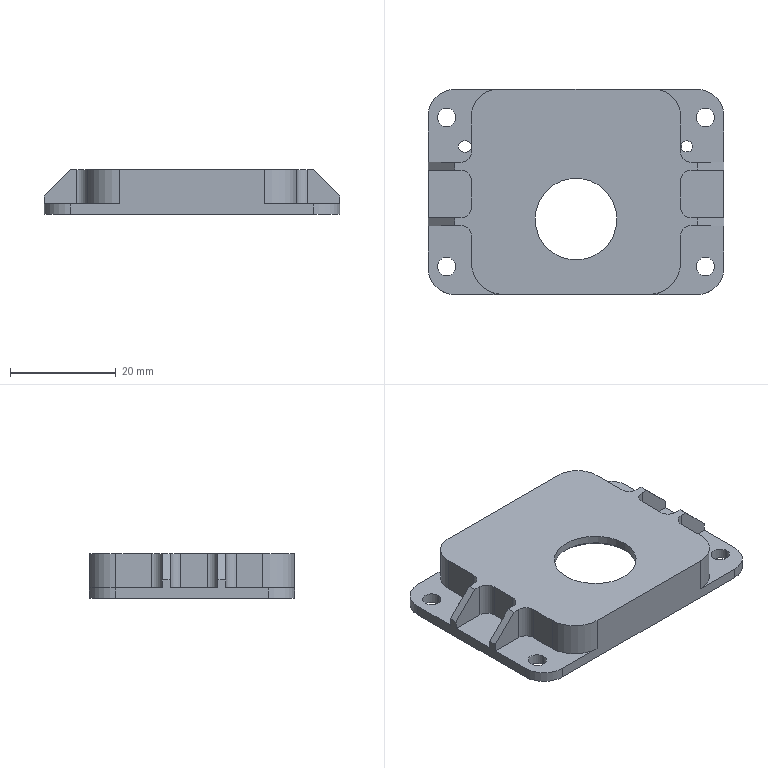NC program | NX | posted with a generic post | part box 56 x 38.85 x 8.5 mm
Lines 1051 to 2659 of 4316:
(CAVITY_MILL_COPY , TOOL : D4)
N2082 T11 M6
N2084 G54
N2086 G17 G0 G90 X-22.6 Y-12.105 S9500 M3
N2088 G43 Z30. H11
N2090 Z0.618
N2092 G94 G1 Z-0.382 F1000.
N2094 X-22.3 Y-11.932
N2096 G3 X-21.8 Y-11.066 R1.
N2098 G1 Y-8.375 F1400.
N2100 X-23.382
N2102 G2 X-24.06 Y-8.257 R2.
N2104 G3 X-25.044 Y-8.434 R1.
N2106 G1 X-25.164 Y-8.535
N2108 Z0.618
N2110 G0 Z30.
N2112 X-22.6 Y-12.201
N2114 Z0.235
N2116 G1 Z-0.765 F1000.
N2118 X-22.3 Y-12.028
N2120 G3 X-21.8 Y-11.162 R1.
N2122 G1 Y-8.375 F1400.
N2124 X-23.765
N2126 G2 X-24.289 Y-8.301 R2.016
N2128 G3 X-25.257 Y-8.551 R1.
N2130 G1 X-25.37 Y-8.662
N2132 Z0.235
N2134 G0 X-22.6 Y-12.258 Z-0.147
N2136 G1 Z-1.147 F1000.
N2138 X-22.3 Y-12.084
N2140 G3 X-21.8 Y-11.218 R1.
N2142 G1 Y-8.375 F1400.
N2144 X-24.147
N2146 G2 X-24.473 Y-8.346 R2.015
N2148 G3 X-25.411 Y-8.693 R1.
N2150 G1 X-25.512 Y-8.814
N2152 Z-0.147
N2154 G0 X-22.6 Y-12.301 Z-0.529
N2156 G1 Z-1.529 F1000.
N2158 X-22.3 Y-12.127
N2160 G3 X-21.8 Y-11.261 R1.
N2162 G1 Y-8.375 F1400.
N2164 X-24.529
N2166 X-24.647 Y-8.372
N2168 G3 X-25.541 Y-8.82 R1.
N2170 G1 X-25.627 Y-8.951
N2172 Z-0.529
N2174 G0 X-22.6 Y-12.311 Z-0.912
N2176 G1 Z-1.912 F1000.
N2178 X-22.3 Y-12.138
N2180 G3 X-21.8 Y-11.272 R1.
N2182 G1 Y-8.375 F1400.
N2184 X-24.697
N2186 G3 X-25.563 Y-8.875 R1.
N2188 G1 X-25.675 Y-9.069
N2190 Z-0.912
N2192 G0 X-22.6 Y-12.311 Z-1.294
N2194 G1 Z-2.294 F1000.
N2196 X-22.3 Y-12.138
N2198 G3 X-21.8 Y-11.272 R1.
N2200 G1 Y-8.375 F1400.
N2202 X-24.697
N2204 G3 X-25.563 Y-8.875 R1.
N2206 G1 X-25.716 Y-9.141
N2208 Z-1.294
N2210 G0 X-22.6 Y-12.311 Z-1.676
N2212 G1 Z-2.676 F1000.
N2214 X-22.3 Y-12.138
N2216 G3 X-21.8 Y-11.272 R1.
N2218 G1 Y-8.375 F1400.
N2220 X-24.697
N2222 G3 X-25.563 Y-8.875 R1.
N2224 G1 X-25.736 Y-9.174
N2226 Z-1.676
N2228 G0 X-22.6 Y-12.311 Z-2.059
N2230 G1 Z-3.059 F1000.
N2232 X-22.3 Y-12.138
N2234 G3 X-21.8 Y-11.272 R1.
N2236 G1 Y-8.375 F1400.
N2238 X-24.697
N2240 G3 X-25.563 Y-8.875 R1.
N2242 G1 X-25.736 Y-9.175
N2244 Z-2.059
N2246 G0 X-22.6 Y-12.311 Z-2.441
N2248 G1 Z-3.441 F1000.
N2250 X-22.3 Y-12.138
N2252 G3 X-21.8 Y-11.272 R1.
N2254 G1 Y-8.375 F1400.
N2256 X-24.697
N2258 G3 X-25.563 Y-8.875 R1.
N2260 G1 X-25.736 Y-9.175
N2262 Z-2.441
N2264 G0 X-22.6 Y-12.311 Z-2.824
N2266 G1 Z-3.824 F1000.
N2268 X-22.3 Y-12.138
N2270 G3 X-21.8 Y-11.272 R1.
N2272 G1 Y-8.375 F1400.
N2274 X-24.697
N2276 G3 X-25.563 Y-8.875 R1.
N2278 G1 X-25.736 Y-9.175
N2280 Z-2.824
N2282 G0 X-22.6 Y-12.311 Z-3.206
N2284 G1 Z-4.206 F1000.
N2286 X-22.3 Y-12.138
N2288 G3 X-21.8 Y-11.272 R1.
N2290 G1 Y-8.375 F1400.
N2292 X-24.697
N2294 G3 X-25.563 Y-8.875 R1.
N2296 G1 X-25.736 Y-9.175
N2298 Z-3.206
N2300 G0 X-22.6 Y-12.311 Z-3.588
N2302 G1 Z-4.588 F1000.
N2304 X-22.3 Y-12.138
N2306 G3 X-21.8 Y-11.272 R1.
N2308 G1 Y-8.375 F1400.
N2310 X-24.697
N2312 G3 X-25.563 Y-8.875 R1.
N2314 G1 X-25.736 Y-9.175
N2316 Z-3.588
N2318 G0 X-22.6 Y-12.311 Z-3.971
N2320 G1 Z-4.971 F1000.
N2322 X-22.3 Y-12.138
N2324 G3 X-21.8 Y-11.272 R1.
N2326 G1 Y-8.375 F1400.
N2328 X-24.697
N2330 G3 X-25.563 Y-8.875 R1.
N2332 G1 X-25.736 Y-9.175
N2334 Z-3.971
N2336 G0 X-22.6 Y-12.311 Z-4.353
N2338 G1 Z-5.353 F1000.
N2340 X-22.3 Y-12.138
N2342 G3 X-21.8 Y-11.272 R1.
N2344 G1 Y-8.375 F1400.
N2346 X-24.697
N2348 G3 X-25.563 Y-8.875 R1.
N2350 G1 X-25.736 Y-9.175
N2352 Z-4.353
N2354 G0 X-22.6 Y-12.311 Z-4.735
N2356 G1 Z-5.735 F1000.
N2358 X-22.3 Y-12.138
N2360 G3 X-21.8 Y-11.272 R1.
N2362 G1 Y-8.375 F1400.
N2364 X-24.697
N2366 G3 X-25.563 Y-8.875 R1.
N2368 G1 X-25.736 Y-9.175
N2370 Z-4.735
N2372 G0 X-22.6 Y-12.311 Z-5.118
N2374 G1 Z-6.118 F1000.
N2376 X-22.3 Y-12.138
N2378 G3 X-21.8 Y-11.272 R1.
N2380 G1 Y-8.375 F1400.
N2382 X-24.697
N2384 G3 X-25.563 Y-8.875 R1.
N2386 G1 X-25.736 Y-9.175
N2388 Z-5.118
N2390 G0 X-22.6 Y-12.311 Z-5.5
N2392 G1 Z-6.5 F1000.
N2394 X-22.3 Y-12.138
N2396 G3 X-21.8 Y-11.272 R1.
N2398 G1 Y-8.375 F1400.
N2400 X-24.697
N2402 G3 X-25.563 Y-8.875 R1.
N2404 G1 X-25.736 Y-9.175
N2406 Z-5.5
N2408 G0 Z30.
N2410 X-25.495 Y-3.037
N2412 Z0.618
N2414 G1 Z-0.382 F1000.
N2416 X-25.36 Y-3.118
N2418 G3 X-24.36 Y-3.13 R1.
N2420 G2 X-23.382 Y-2.875 R2. F1400.
N2422 G1 X-21.8
N2424 Y2.125
N2426 X-23.382
N2428 G2 X-24.361 Y2.381 R2.
N2430 G3 X-25.361 Y2.369 R1.
N2432 G1 X-25.496 Y2.289
N2434 Z0.618
N2436 G0 Z30.
N2438 X-25.877 Y-3.037
N2440 Z0.235
N2442 G1 Z-0.765 F1000.
N2444 X-25.742 Y-3.118
N2446 G3 X-24.742 Y-3.13 R1.
N2448 G2 X-23.765 Y-2.875 R2. F1400.
N2450 G1 X-21.8
N2452 Y2.125
N2454 X-23.765
N2456 G2 X-24.744 Y2.381 R2.
N2458 G3 X-25.744 Y2.369 R1.
N2460 G1 X-25.878 Y2.289
N2462 Z0.235
N2464 G0 X-25.545 Y1.215 Z-0.147
N2466 G1 Z-1.147 F1000.
N2468 X-24.284 Y0.498
N2470 G2 X-23.779 Y-0.365 R1.
N2472 X-24.94 Y-2.525 R2.56 F1400.
N2474 G3 X-25.129 Y-3.133 R0.5
N2476 G2 X-24.147 Y-2.875 R2.
N2478 G1 X-21.8
N2480 Y2.125
N2482 X-24.147
N2484 G2 X-25.159 Y2.4 R2.
N2486 G3 X-24.967 Y1.781 R0.5
N2488 G2 X-23.779 Y-0.365 R2.56
N2490 X-24.273 Y-1.234 R1.
N2492 G1 X-25.524 Y-1.967
N2494 Z-0.147
N2496 G0 X-25.927 Y1.215 Z-0.529
N2498 G1 Z-1.529 F1000.
N2500 X-24.666 Y0.496
N2502 G2 X-24.161 Y-0.367 R1.
N2504 X-25.322 Y-2.525 R2.56 F1400.
N2506 G3 X-25.512 Y-3.133 R0.5
N2508 G2 X-24.529 Y-2.875 R2.
N2510 G1 X-21.8
N2512 Y2.125
N2514 X-24.529
N2516 G2 X-25.541 Y2.4 R2.
N2518 G3 X-25.35 Y1.781 R0.5
N2520 G2 X-24.161 Y-0.367 R2.56
N2522 X-24.656 Y-1.236 R1.
N2524 G1 X-25.906 Y-1.967
N2526 Z-0.529
N2528 G0 X-26.31 Y1.216 Z-0.912
N2530 G1 Z-1.912 F1000.
N2532 X-25.048 Y0.495
N2534 G2 X-24.544 Y-0.369 R1.
N2536 X-25.705 Y-2.525 R2.56 F1400.
N2538 G3 X-25.894 Y-3.133 R0.5
N2540 G2 X-24.912 Y-2.875 R2.
N2542 G1 X-21.8
N2544 Y2.125
N2546 X-24.912
N2548 G2 X-25.924 Y2.4 R2.
N2550 G3 X-25.732 Y1.781 R0.5
N2552 G2 X-24.544 Y-0.369 R2.56
N2554 X-25.039 Y-1.237 R1.
N2556 G1 X-26.289 Y-1.966
N2558 Z-0.912
N2560 G0 X-26.693 Y1.216 Z-1.294
N2562 G1 Z-2.294 F1000.
N2564 X-25.43 Y0.494
N2566 G2 X-24.926 Y-0.37 R1.
N2568 X-26.087 Y-2.525 R2.56 F1400.
N2570 G3 X-26.276 Y-3.133 R0.5
N2572 G2 X-25.294 Y-2.875 R2.
N2574 G1 X-21.8
N2576 Y2.125
N2578 X-25.294
N2580 G2 X-26.306 Y2.4 R2.
N2582 G3 X-26.114 Y1.781 R0.5
N2584 G2 X-24.926 Y-0.37 R2.56
N2586 X-25.422 Y-1.238 R1.
N2588 G1 X-26.671 Y-1.966
N2590 Z-1.294
N2592 G0 X-27.075 Y1.216 Z-1.676
N2594 G1 Z-2.676 F1000.
N2596 X-25.811 Y0.493
N2598 G2 X-25.308 Y-0.372 R1.
N2600 X-26.469 Y-2.525 R2.56 F1400.
N2602 G3 X-26.659 Y-3.133 R0.5
N2604 G2 X-25.676 Y-2.875 R2.
N2606 G1 X-21.8
N2608 Y2.125
N2610 X-25.676
N2612 G2 X-26.688 Y2.4 R2.
N2614 G3 X-26.497 Y1.781 R0.5
N2616 G2 X-25.308 Y-0.372 R2.56
N2618 X-25.805 Y-1.239 R1.
N2620 G1 X-27.053 Y-1.966
N2622 Z-1.676
N2624 G0 X-27.448 Y-1.973 Z-2.059
N2626 G1 Z-3.059 F1000.
N2628 X-26.188 Y-1.24
N2630 G3 X-25.691 Y-0.373 R1.
N2632 G1 X-23.891 Y-0.367
N2634 G2 X-23.946 Y-1.075 R4.36 F1400.
N2636 G1 X-23.6
N2638 Y0.325
N2640 X-23.948
N2642 G2 X-23.891 Y-0.367 R4.36
N2644 G1 X-25.691 Y-0.373
N2646 G2 X-26.866 Y-2.534 R2.56
N2648 G3 X-27.055 Y-3.151 R0.5
N2650 G2 X-26.007 Y-2.875 R2.026
N2652 G1 X-21.8
N2654 Y2.125
N2656 X-26.029
N2658 G2 X-27.08 Y2.412 R2.015
N2660 G3 X-26.888 Y1.786 R0.5
N2662 G2 X-25.691 Y-0.373 R2.56
N2664 X-26.188 Y-1.24 R1.
N2666 G1 X-27.448 Y-1.973
N2668 Z-2.059
N2670 G0 X-27.817 Y-1.965 Z-2.441
N2672 G1 Z-3.441 F1000.
N2674 X-26.572 Y-1.244
N2676 G3 X-26.073 Y-0.377 R1.
N2678 G1 X-24.273 Y-0.375
N2680 G2 X-24.329 Y-1.075 R4.36 F1400.
N2682 G1 X-23.6
N2684 Y0.325
N2686 X-24.331
N2688 G2 X-24.273 Y-0.375 R4.36
N2690 G1 X-26.073 Y-0.377
N2692 G2 X-27.234 Y-2.525 R2.56
N2694 G3 X-27.424 Y-3.133 R0.5
N2696 G2 X-26.441 Y-2.875 R2.
N2698 G1 X-21.8
N2700 Y2.125
N2702 X-26.441
N2704 G2 X-27.453 Y2.4 R2.
N2706 G3 X-27.261 Y1.781 R0.5
N2708 G2 X-26.073 Y-0.377 R2.56
N2710 X-26.572 Y-1.244 R1.
N2712 G1 X-27.817 Y-1.965
N2714 Z-2.441
N2716 G0 X-28.199 Z-2.824
N2718 G1 Z-3.824 F1000.
N2720 X-26.954 Y-1.244
N2722 G3 X-26.455 Y-0.377 R1.
N2724 G1 X-24.655 Y-0.375
N2726 G2 X-24.711 Y-1.075 R4.36 F1400.
N2728 G1 X-23.6
N2730 Y0.325
N2732 X-24.713
N2734 G2 X-24.655 Y-0.375 R4.36
N2736 G1 X-26.455 Y-0.377
N2738 G2 X-27.616 Y-2.525 R2.56
N2740 G3 X-27.806 Y-3.133 R0.5
N2742 G2 X-26.824 Y-2.875 R2.
N2744 G1 X-21.8
N2746 Y2.125
N2748 X-26.824
N2750 G2 X-27.835 Y2.4 R2.
N2752 G3 X-27.644 Y1.781 R0.5
N2754 G2 X-26.455 Y-0.377 R2.56
N2756 X-26.954 Y-1.244 R1.
N2758 G1 X-28.199 Y-1.965
N2760 Z-2.824
N2762 G0 X-28.581 Z-3.206
N2764 G1 Z-4.206 F1000.
N2766 X-27.337 Y-1.245
N2768 G3 X-26.838 Y-0.378 R1.
N2770 G1 X-24.438 Y-0.375
N2772 X-24.439 Y-0.475 F1400.
N2774 X-24.2
N2776 Y-0.275
N2778 X-24.439
N2780 X-24.438 Y-0.375
N2782 X-26.838 Y-0.378
N2784 Y-0.43
N2786 G2 X-27.999 Y-2.525 R2.56
N2788 G3 X-28.188 Y-3.133 R0.5
N2790 G2 X-27.206 Y-2.875 R2.
N2792 G1 X-21.8
N2794 Y2.125
N2796 X-27.206
N2798 G2 X-28.218 Y2.4 R2.
N2800 G3 X-28.026 Y1.781 R0.5
N2802 G2 X-26.838 Y-0.378 R2.56
N2804 X-27.337 Y-1.245 R1.
N2806 G1 X-28.581 Y-1.965
N2808 Z-3.206
N2810 G0 X-28.964 Z-3.588
N2812 G1 Z-4.588 F1000.
N2814 X-27.719 Y-1.245
N2816 G3 X-27.22 Y-0.378 R1.
N2818 G1 X-24.82 Y-0.375
N2820 X-24.821 Y-0.475 F1400.
N2822 X-24.2
N2824 Y-0.275
N2826 X-24.821
N2828 X-24.82 Y-0.375
N2830 X-27.22 Y-0.378
N2832 Y-0.43
N2834 G2 X-28.381 Y-2.525 R2.56
N2836 G3 X-28.571 Y-3.133 R0.5
N2838 G2 X-27.588 Y-2.875 R2.
N2840 G1 X-21.8
N2842 Y2.125
N2844 X-27.588
N2846 G2 X-28.6 Y2.4 R2.
N2848 G3 X-28.409 Y1.781 R0.5
N2850 G2 X-27.22 Y-0.378 R2.56
N2852 X-27.719 Y-1.245 R1.
N2854 G1 X-28.964 Y-1.965
N2856 Z-3.588
N2858 G0 X-29.347 Y-1.966 Z-3.971
N2860 G1 Z-4.971 F1000.
N2862 X-28.103 Y-1.245
N2864 G3 X-27.604 Y-0.378 R1.
N2866 G1 X-25.204 Y-0.375
N2868 X-25.205 Y-0.475 F1400.
N2870 X-24.2
N2872 Y-0.275
N2874 X-25.206
N2876 X-25.204 Y-0.375
N2878 X-27.604 Y-0.378
N2880 X-27.605 Y-0.43
N2882 G2 X-28.764 Y-2.525 R2.56
N2884 G3 X-28.954 Y-3.133 R0.5
N2886 G2 X-27.971 Y-2.875 R2.
N2888 G1 X-21.8
N2890 Y2.125
N2892 X-27.971
N2894 G2 X-28.958 Y2.386 R2.
N2896 G3 X-28.772 Y1.778 R0.5
N2898 G2 X-28.136 Y1.18 R2.56
N2900 X-27.604 Y-0.378 R2.56
N2902 X-28.103 Y-1.245 R1.
N2904 G1 X-29.347 Y-1.966
N2906 Z-3.971
N2908 G0 X-29.384 Y-1.969 Z-4.353
N2910 G1 Z-5.353 F1000.
N2912 X-28.143 Y-1.248
N2914 G3 X-27.645 Y-0.381 R1.
N2916 G1 X-25.245 Y-0.375
N2918 X-25.246 Y-0.475 F1400.
N2920 X-24.2
N2922 Y-0.275
N2924 X-25.247
N2926 X-25.245 Y-0.375
N2928 X-27.645 Y-0.381
N2930 X-27.646 Y-0.433
N2932 G2 X-28.8 Y-2.527 R2.56
N2934 G3 X-28.988 Y-3.136 R0.5
N2936 G2 X-28. Y-2.875 R2.
N2938 G1 X-21.8
N2940 Y2.125
N2942 X-28.
N2944 G2 X-29.02 Y2.404 R2.
N2946 G3 X-28.843 Y1.793 R0.5
N2948 G2 X-28.677 Y1.669 R2.56
N2950 G1 X-28.595 Y1.602
N2952 G2 X-27.645 Y-0.381 R2.56
N2954 X-28.143 Y-1.248 R1.
N2956 G1 X-29.384 Y-1.969
N2958 Z-4.353
N2960 G0 Z-4.735
N2962 G1 Z-5.735 F1000.
N2964 X-28.143 Y-1.248
N2966 G3 X-27.645 Y-0.381 R1.
N2968 G1 X-25.245 Y-0.375
N2970 X-25.246 Y-0.475 F1400.
N2972 X-24.2
N2974 Y-0.275
N2976 X-25.247
N2978 X-25.245 Y-0.375
N2980 X-27.645 Y-0.381
N2982 X-27.646 Y-0.433
N2984 G2 X-28.8 Y-2.527 R2.56
N2986 G3 X-28.988 Y-3.136 R0.5
N2988 G2 X-28. Y-2.875 R2.
N2990 G1 X-21.8
N2992 Y2.125
N2994 X-28.
N2996 G2 X-29.02 Y2.404 R2.
N2998 G3 X-28.843 Y1.793 R0.5
N3000 G2 X-28.677 Y1.669 R2.56
N3002 G1 X-28.595 Y1.602
N3004 G2 X-27.645 Y-0.381 R2.56
N3006 X-28.143 Y-1.248 R1.
N3008 G1 X-29.384 Y-1.969
N3010 Z-4.735
N3012 G0 Z-5.118
N3014 G1 Z-6.118 F1000.
N3016 X-28.143 Y-1.248
N3018 G3 X-27.645 Y-0.381 R1.
N3020 G1 X-25.245 Y-0.375
N3022 X-25.246 Y-0.475 F1400.
N3024 X-24.2
N3026 Y-0.275
N3028 X-25.247
N3030 X-25.245 Y-0.375
N3032 X-27.645 Y-0.381
N3034 X-27.646 Y-0.433
N3036 G2 X-28.8 Y-2.527 R2.56
N3038 G3 X-28.988 Y-3.136 R0.5
N3040 G2 X-28. Y-2.875 R2.
N3042 G1 X-21.8
N3044 Y2.125
N3046 X-28.
N3048 G2 X-29.02 Y2.404 R2.
N3050 G3 X-28.843 Y1.793 R0.5
N3052 G2 X-28.677 Y1.669 R2.56
N3054 G1 X-28.595 Y1.602
N3056 G2 X-27.645 Y-0.381 R2.56
N3058 X-28.143 Y-1.248 R1.
N3060 G1 X-29.384 Y-1.969
N3062 Z-5.118
N3064 G0 Z-5.5
N3066 G1 Z-6.5 F1000.
N3068 X-28.143 Y-1.248
N3070 G3 X-27.645 Y-0.381 R1.
N3072 G1 X-25.245 Y-0.375
N3074 X-25.246 Y-0.475 F1400.
N3076 X-24.2
N3078 Y-0.275
N3080 X-25.247
N3082 X-25.245 Y-0.375
N3084 X-27.645 Y-0.381
N3086 X-27.646 Y-0.433
N3088 G2 X-28.8 Y-2.527 R2.56
N3090 G3 X-28.988 Y-3.136 R0.5
N3092 G2 X-28. Y-2.875 R2.
N3094 G1 X-21.8
N3096 Y2.125
N3098 X-28.
N3100 G2 X-29.02 Y2.404 R2.
N3102 G3 X-28.843 Y1.793 R0.5
N3104 G2 X-28.677 Y1.669 R2.56
N3106 G1 X-28.595 Y1.602
N3108 G2 X-27.645 Y-0.381 R2.56
N3110 X-28.143 Y-1.248 R1.
N3112 G1 X-29.384 Y-1.969
N3114 Z-5.5
N3116 G0 Z30.
N3118 X-25.164 Y7.785
N3120 Z0.618
N3122 G1 Z-0.382 F1000.
N3124 X-25.044 Y7.684
N3126 G3 X-24.06 Y7.507 R1.
N3128 G2 X-23.382 Y7.625 R2. F1400.
N3130 G1 X-21.8
N3132 Y10.316
N3134 G3 X-22.3 Y11.182 R1.
N3136 G1 X-22.6 Y11.355
N3138 Z0.618
N3140 G0 Z30.
N3142 X-25.367 Y7.921
N3144 Z0.235
N3146 G1 Z-0.765 F1000.
N3148 X-25.256 Y7.811
N3150 G3 X-24.289 Y7.555 R1.
N3152 G2 X-23.765 Y7.625 R2. F1400.
N3154 G1 X-21.8
N3156 Y10.412
N3158 G3 X-22.3 Y11.278 R1.
N3160 G1 X-22.6 Y11.451
N3162 Z0.235
N3164 G0 X-25.509 Y8.071 Z-0.147
N3166 G1 Z-1.147 F1000.
N3168 X-25.41 Y7.95
N3170 G3 X-24.474 Y7.598 R1.
N3172 G2 X-24.147 Y7.625 R2. F1400.
N3174 G1 X-21.8
N3176 Y10.469
N3178 G3 X-22.3 Y11.335 R1.
N3180 G1 X-22.6 Y11.508
N3182 Z-0.147
N3184 G0 X-25.628 Y8.201 Z-0.529
N3186 G1 Z-1.529 F1000.
N3188 X-25.541 Y8.07
N3190 G3 X-24.647 Y7.622 R1.
N3192 G1 X-24.529 Y7.625 F1400.
N3194 X-21.8
N3196 Y10.512
N3198 G3 X-22.3 Y11.378 R1.
N3200 G1 X-22.6 Y11.551
N3202 Z-0.529
N3204 G0 X-25.675 Y8.319 Z-0.912
N3206 G1 Z-1.912 F1000.
N3208 X-25.563 Y8.125
N3210 G3 X-24.697 Y7.625 R1.
N3212 G1 X-21.8 F1400.
N3214 Y10.522
N3216 G3 X-22.3 Y11.388 R1.
N3218 G1 X-22.6 Y11.561
N3220 Z-0.912
N3222 G0 X-25.718 Y8.393 Z-1.294
N3224 G1 Z-2.294 F1000.
N3226 X-25.563 Y8.125
N3228 G3 X-24.697 Y7.625 R1.
N3230 G1 X-21.8 F1400.
N3232 Y10.522
N3234 G3 X-22.3 Y11.388 R1.
N3236 G1 X-22.6 Y11.561
N3238 Z-1.294
N3240 G0 X-25.736 Y8.424 Z-1.676
N3242 G1 Z-2.676 F1000.
N3244 X-25.563 Y8.125
N3246 G3 X-24.697 Y7.625 R1.
N3248 G1 X-21.8 F1400.
N3250 Y10.522
N3252 G3 X-22.3 Y11.388 R1.
N3254 G1 X-22.6 Y11.561
N3256 Z-1.676
N3258 G0 X-25.736 Y8.425 Z-2.059
N3260 G1 Z-3.059 F1000.
N3262 X-25.563 Y8.125
N3264 G3 X-24.697 Y7.625 R1.
N3266 G1 X-21.8 F1400.
N3268 Y10.522
N3270 G3 X-22.3 Y11.388 R1.
N3272 G1 X-22.6 Y11.561
N3274 Z-2.059
N3276 G0 X-25.736 Y8.425 Z-2.441
N3278 G1 Z-3.441 F1000.
N3280 X-25.563 Y8.125
N3282 G3 X-24.697 Y7.625 R1.
N3284 G1 X-21.8 F1400.
N3286 Y10.522
N3288 G3 X-22.3 Y11.388 R1.
N3290 G1 X-22.6 Y11.561
N3292 Z-2.441
N3294 G0 X-25.736 Y8.425 Z-2.824
N3296 G1 Z-3.824 F1000.
N3298 X-25.563 Y8.125
N3300 G3 X-24.697 Y7.625 R1.
N3302 G1 X-21.8 F1400.
N3304 Y10.522
N3306 G3 X-22.3 Y11.388 R1.
N3308 G1 X-22.6 Y11.561
N3310 Z-2.824
N3312 G0 X-25.736 Y8.425 Z-3.206
N3314 G1 Z-4.206 F1000.
N3316 X-25.563 Y8.125
N3318 G3 X-24.697 Y7.625 R1.
N3320 G1 X-21.8 F1400.
N3322 Y10.522
N3324 G3 X-22.3 Y11.388 R1.
N3326 G1 X-22.6 Y11.561
N3328 Z-3.206
N3330 G0 X-25.736 Y8.425 Z-3.588
N3332 G1 Z-4.588 F1000.
N3334 X-25.563 Y8.125
N3336 G3 X-24.697 Y7.625 R1.
N3338 G1 X-21.8 F1400.
N3340 Y10.522
N3342 G3 X-22.3 Y11.388 R1.
N3344 G1 X-22.6 Y11.561
N3346 Z-3.588
N3348 G0 X-25.736 Y8.425 Z-3.971
N3350 G1 Z-4.971 F1000.
N3352 X-25.563 Y8.125
N3354 G3 X-24.697 Y7.625 R1.
N3356 G1 X-21.8 F1400.
N3358 Y10.522
N3360 G3 X-22.3 Y11.388 R1.
N3362 G1 X-22.6 Y11.561
N3364 Z-3.971
N3366 G0 X-25.736 Y8.425 Z-4.353
N3368 G1 Z-5.353 F1000.
N3370 X-25.563 Y8.125
N3372 G3 X-24.697 Y7.625 R1.
N3374 G1 X-21.8 F1400.
N3376 Y10.522
N3378 G3 X-22.3 Y11.388 R1.
N3380 G1 X-22.6 Y11.561
N3382 Z-4.353
N3384 G0 X-25.736 Y8.425 Z-4.735
N3386 G1 Z-5.735 F1000.
N3388 X-25.563 Y8.125
N3390 G3 X-24.697 Y7.625 R1.
N3392 G1 X-21.8 F1400.
N3394 Y10.522
N3396 G3 X-22.3 Y11.388 R1.
N3398 G1 X-22.6 Y11.561
N3400 Z-4.735
N3402 G0 X-25.736 Y8.425 Z-5.118
N3404 G1 Z-6.118 F1000.
N3406 X-25.563 Y8.125
N3408 G3 X-24.697 Y7.625 R1.
N3410 G1 X-21.8 F1400.
N3412 Y10.522
N3414 G3 X-22.3 Y11.388 R1.
N3416 G1 X-22.6 Y11.561
N3418 Z-5.118
N3420 G0 X-25.736 Y8.425 Z-5.5
N3422 G1 Z-6.5 F1000.
N3424 X-25.563 Y8.125
N3426 G3 X-24.697 Y7.625 R1.
N3428 G1 X-21.8 F1400.
N3430 Y10.522
N3432 G3 X-22.3 Y11.388 R1.
N3434 G1 X-22.6 Y11.561
N3436 Z-5.5
N3438 G0 Z30.
N3440 X22.6 Y11.355
N3442 Z0.618
N3444 G1 Z-0.382 F1000.
N3446 X22.3 Y11.182
N3448 G3 X21.8 Y10.316 R1.
N3450 G1 Y7.625 F1400.
N3452 X23.382
N3454 G2 X24.06 Y7.507 R2.
N3456 G3 X25.044 Y7.684 R1.
N3458 G1 X25.164 Y7.785
N3460 Z0.618
N3462 G0 Z30.
N3464 X22.6 Y11.451
N3466 Z0.235
N3468 G1 Z-0.765 F1000.
N3470 X22.3 Y11.278
N3472 G3 X21.8 Y10.412 R1.
N3474 G1 Y7.625 F1400.
N3476 X23.765
N3478 G2 X24.289 Y7.555 R2.
N3480 G3 X25.256 Y7.811 R1.
N3482 G1 X25.367 Y7.921
N3484 Z0.235
N3486 G0 X22.6 Y11.508 Z-0.147
N3488 G1 Z-1.147 F1000.
N3490 X22.3 Y11.335
N3492 G3 X21.8 Y10.469 R1.
N3494 G1 Y7.625 F1400.
N3496 X24.147
N3498 G2 X24.474 Y7.598 R2.
N3500 G3 X25.41 Y7.95 R1.
N3502 G1 X25.509 Y8.071
N3504 Z-0.147
N3506 G0 X22.6 Y11.551 Z-0.529
N3508 G1 Z-1.529 F1000.
N3510 X22.3 Y11.378
N3512 G3 X21.8 Y10.512 R1.
N3514 G1 Y7.625 F1400.
N3516 X24.529
N3518 X24.647 Y7.622
N3520 G3 X25.541 Y8.07 R1.
N3522 G1 X25.628 Y8.201
N3524 Z-0.529
N3526 G0 X22.6 Y11.561 Z-0.912
N3528 G1 Z-1.912 F1000.
N3530 X22.3 Y11.388
N3532 G3 X21.8 Y10.522 R1.
N3534 G1 Y7.625 F1400.
N3536 X24.697
N3538 G3 X25.563 Y8.125 R1.
N3540 G1 X25.675 Y8.319
N3542 Z-0.912
N3544 G0 X22.6 Y11.561 Z-1.294
N3546 G1 Z-2.294 F1000.
N3548 X22.3 Y11.388
N3550 G3 X21.8 Y10.522 R1.
N3552 G1 Y7.625 F1400.
N3554 X24.697
N3556 G3 X25.563 Y8.125 R1.
N3558 G1 X25.718 Y8.393
N3560 Z-1.294
N3562 G0 X22.6 Y11.561 Z-1.676
N3564 G1 Z-2.676 F1000.
N3566 X22.3 Y11.388
N3568 G3 X21.8 Y10.522 R1.
N3570 G1 Y7.625 F1400.
N3572 X24.697
N3574 G3 X25.563 Y8.125 R1.
N3576 G1 X25.736 Y8.424
N3578 Z-1.676
N3580 G0 X22.6 Y11.561 Z-2.059
N3582 G1 Z-3.059 F1000.
N3584 X22.3 Y11.388
N3586 G3 X21.8 Y10.522 R1.
N3588 G1 Y7.625 F1400.
N3590 X24.697
N3592 G3 X25.563 Y8.125 R1.
N3594 G1 X25.736 Y8.425
N3596 Z-2.059
N3598 G0 X22.6 Y11.561 Z-2.441
N3600 G1 Z-3.441 F1000.
N3602 X22.3 Y11.388
N3604 G3 X21.8 Y10.522 R1.
N3606 G1 Y7.625 F1400.
N3608 X24.697
N3610 G3 X25.563 Y8.125 R1.
N3612 G1 X25.736 Y8.425
N3614 Z-2.441
N3616 G0 X22.6 Y11.561 Z-2.824
N3618 G1 Z-3.824 F1000.
N3620 X22.3 Y11.388
N3622 G3 X21.8 Y10.522 R1.
N3624 G1 Y7.625 F1400.
N3626 X24.697
N3628 G3 X25.563 Y8.125 R1.
N3630 G1 X25.736 Y8.425
N3632 Z-2.824
N3634 G0 X22.6 Y11.561 Z-3.206
N3636 G1 Z-4.206 F1000.
N3638 X22.3 Y11.388
N3640 G3 X21.8 Y10.522 R1.
N3642 G1 Y7.625 F1400.
N3644 X24.697
N3646 G3 X25.563 Y8.125 R1.
N3648 G1 X25.736 Y8.425
N3650 Z-3.206
N3652 G0 X22.6 Y11.561 Z-3.588
N3654 G1 Z-4.588 F1000.
N3656 X22.3 Y11.388
N3658 G3 X21.8 Y10.522 R1.
N3660 G1 Y7.625 F1400.
N3662 X24.697
N3664 G3 X25.563 Y8.125 R1.
N3666 G1 X25.736 Y8.425
N3668 Z-3.588
N3670 G0 X22.6 Y11.561 Z-3.971
N3672 G1 Z-4.971 F1000.
N3674 X22.3 Y11.388
N3676 G3 X21.8 Y10.522 R1.
N3678 G1 X21.801 Y7.625 F1400.
N3680 X24.697
N3682 G3 X25.563 Y8.125 R1.
N3684 G1 X25.736 Y8.425
N3686 Z-3.971
N3688 G0 X22.6 Y11.561 Z-4.353
N3690 G1 Z-5.353 F1000.
N3692 X22.3 Y11.388
N3694 G3 X21.8 Y10.522 R1.
N3696 G1 X21.801 Y7.625 F1400.
N3698 X24.697
N3700 G3 X25.563 Y8.125 R1.
N3702 G1 X25.736 Y8.425
N3704 Z-4.353
N3706 G0 X22.6 Y11.561 Z-4.735
N3708 G1 Z-5.735 F1000.
N3710 X22.3 Y11.388
N3712 G3 X21.8 Y10.522 R1.
N3714 G1 X21.801 Y7.625 F1400.
N3716 X24.697
N3718 G3 X25.563 Y8.125 R1.
N3720 G1 X25.736 Y8.425
N3722 Z-4.735
N3724 G0 X22.6 Y11.561 Z-5.118
N3726 G1 Z-6.118 F1000.
N3728 X22.3 Y11.388
N3730 G3 X21.8 Y10.522 R1.
N3732 G1 X21.801 Y7.625 F1400.
N3734 X24.697
N3736 G3 X25.563 Y8.125 R1.
N3738 G1 X25.736 Y8.425
N3740 Z-5.118
N3742 G0 X22.6 Y11.561 Z-5.5
N3744 G1 Z-6.5 F1000.
N3746 X22.3 Y11.388
N3748 G3 X21.8 Y10.522 R1.
N3750 G1 X21.801 Y7.625 F1400.
N3752 X24.697
N3754 G3 X25.563 Y8.125 R1.
N3756 G1 X25.736 Y8.425
N3758 Z-5.5
N3760 G0 Z30.
N3762 X25.495 Y2.287
N3764 Z0.618
N3766 G1 Z-0.382 F1000.
N3768 X25.36 Y2.367
N3770 G3 X24.36 Y2.38 R1.
N3772 G2 X23.382 Y2.125 R2. F1400.
N3774 G1 X21.8
N3776 Y-2.875
N3778 X23.382
N3780 G2 X24.361 Y-3.131 R2.
N3782 G3 X25.361 Y-3.119 R1.
N3784 G1 X25.496 Y-3.039
N3786 Z0.618
N3788 G0 Z30.
N3790 X25.877 Y2.287
N3792 Z0.235
N3794 G1 Z-0.765 F1000.
N3796 X25.742 Y2.367
N3798 G3 X24.742 Y2.38 R1.
N3800 G2 X23.765 Y2.125 R2. F1400.
N3802 G1 X21.8
N3804 Y-2.875
N3806 X23.765
N3808 G2 X24.744 Y-3.131 R2.
N3810 G3 X25.744 Y-3.119 R1.
N3812 G1 X25.878 Y-3.039
N3814 Z0.235
N3816 G0 X25.545 Y-1.965 Z-0.147
N3818 G1 Z-1.147 F1000.
N3820 X24.284 Y-1.248
N3822 G2 X23.779 Y-0.385 R1.
N3824 X24.94 Y1.775 R2.56 F1400.
N3826 G3 X25.129 Y2.383 R0.5
N3828 G2 X24.147 Y2.125 R2.
N3830 G1 X21.8
N3832 Y-2.875
N3834 X24.147
N3836 G2 X25.159 Y-3.15 R2.
N3838 G3 X24.967 Y-2.531 R0.5
N3840 G2 X23.779 Y-0.385 R2.56
N3842 X24.273 Y0.484 R1.
N3844 G1 X25.524 Y1.217
N3846 Z-0.147
N3848 G0 X25.927 Y-1.965 Z-0.529
N3850 G1 Z-1.529 F1000.
N3852 X24.666 Y-1.246
N3854 G2 X24.161 Y-0.383 R1.
N3856 X25.322 Y1.775 R2.56 F1400.
N3858 G3 X25.512 Y2.383 R0.5
N3860 G2 X24.529 Y2.125 R2.
N3862 G1 X21.8
N3864 Y-2.875
N3866 X24.529
N3868 G2 X25.541 Y-3.15 R2.
N3870 G3 X25.35 Y-2.531 R0.5
N3872 G2 X24.161 Y-0.383 R2.56
N3874 X24.656 Y0.486 R1.
N3876 G1 X25.906 Y1.217
N3878 Z-0.529
N3880 G0 X26.31 Y-1.966 Z-0.912
N3882 G1 Z-1.912 F1000.
N3884 X25.048 Y-1.245
N3886 G2 X24.544 Y-0.381 R1.
N3888 X25.705 Y1.775 R2.56 F1400.
N3890 G3 X25.894 Y2.383 R0.5
N3892 G2 X24.912 Y2.125 R2.
N3894 G1 X21.8
N3896 Y-2.875
N3898 X24.912
N3900 G2 X25.924 Y-3.15 R2.
N3902 G3 X25.732 Y-2.531 R0.5
N3904 G2 X24.544 Y-0.381 R2.56
N3906 X25.039 Y0.487 R1.
N3908 G1 X26.289 Y1.216
N3910 Z-0.912
N3912 G0 X26.693 Y-1.966 Z-1.294
N3914 G1 Z-2.294 F1000.
N3916 X25.43 Y-1.244
N3918 G2 X24.926 Y-0.38 R1.
N3920 X26.087 Y1.775 R2.56 F1400.
N3922 G3 X26.276 Y2.383 R0.5
N3924 G2 X25.294 Y2.125 R2.
N3926 G1 X21.8
N3928 Y-2.875
N3930 X25.294
N3932 G2 X26.306 Y-3.15 R2.
N3934 G3 X26.114 Y-2.531 R0.5
N3936 G2 X24.926 Y-0.38 R2.56
N3938 X25.422 Y0.488 R1.
N3940 G1 X26.671 Y1.216
N3942 Z-1.294
N3944 G0 X27.075 Y-1.966 Z-1.676
N3946 G1 Z-2.676 F1000.
N3948 X25.811 Y-1.243
N3950 G2 X25.308 Y-0.378 R1.
N3952 X26.469 Y1.775 R2.56 F1400.
N3954 G3 X26.659 Y2.383 R0.5
N3956 G2 X25.676 Y2.125 R2.
N3958 G1 X21.8
N3960 Y-2.875
N3962 X25.676
N3964 G2 X26.688 Y-3.15 R2.
N3966 G3 X26.497 Y-2.531 R0.5
N3968 G2 X25.308 Y-0.378 R2.56
N3970 X25.805 Y0.489 R1.
N3972 G1 X27.053 Y1.216
N3974 Z-1.676
N3976 G0 X27.442 Y1.22 Z-2.059
N3978 G1 Z-3.059 F1000.
N3980 X26.188 Y0.49
N3982 G3 X25.691 Y-0.377 R1.
N3984 G1 X23.891 Y-0.383
N3986 G2 X23.946 Y0.325 R4.36 F1400.
N3988 G1 X23.6
N3990 Y-1.075
N3992 X23.948
N3994 G2 X23.891 Y-0.383 R4.36
N3996 G1 X25.691 Y-0.377
N3998 G2 X26.86 Y1.78 R2.56
N4000 G3 X27.049 Y2.393 R0.5
N4002 G2 X26.029 Y2.125 R2.015
N4004 G1 X21.8
N4006 Y-2.875
N4008 X26.007
N4010 G2 X27.087 Y-3.171 R2.026
N4012 G3 X26.895 Y-2.541 R0.5
N4014 G2 X25.691 Y-0.377 R2.56
N4016 X26.188 Y0.49 R1.
N4018 G1 X27.442 Y1.22
N4020 Z-2.059
N4022 G0 X27.817 Y1.215 Z-2.441
N4024 G1 Z-3.441 F1000.
N4026 X26.572 Y0.494
N4028 G3 X26.073 Y-0.373 R1.
N4030 G1 X24.273 Y-0.375
N4032 G2 X24.329 Y0.325 R4.36 F1400.
N4034 G1 X23.6
N4036 Y-1.075
N4038 X24.331
N4040 G2 X24.273 Y-0.375 R4.36
N4042 G1 X26.073 Y-0.373
N4044 G2 X27.234 Y1.775 R2.56
N4046 G3 X27.424 Y2.383 R0.5
N4048 G2 X26.441 Y2.125 R2.
N4050 G1 X21.8
N4052 Y-2.875
N4054 X26.441
N4056 G2 X27.453 Y-3.15 R2.
N4058 G3 X27.261 Y-2.531 R0.5
N4060 G2 X26.073 Y-0.373 R2.56
N4062 X26.572 Y0.494 R1.
N4064 G1 X27.817 Y1.215
N4066 Z-2.441
N4068 G0 X28.199 Z-2.824
N4070 G1 Z-3.824 F1000.
N4072 X26.954 Y0.494
N4074 G3 X26.455 Y-0.373 R1.
N4076 G1 X24.655 Y-0.375
N4078 G2 X24.711 Y0.325 R4.36 F1400.
N4080 G1 X23.6
N4082 Y-1.075
N4084 X24.713
N4086 G2 X24.655 Y-0.375 R4.36
N4088 G1 X26.455 Y-0.373
N4090 G2 X27.616 Y1.775 R2.56
N4092 G3 X27.806 Y2.383 R0.5
N4094 G2 X26.824 Y2.125 R2.
N4096 G1 X21.8
N4098 Y-2.875
N4100 X26.824
N4102 G2 X27.835 Y-3.15 R2.
N4104 G3 X27.644 Y-2.531 R0.5
N4106 G2 X26.455 Y-0.373 R2.56
N4108 X26.954 Y0.494 R1.
N4110 G1 X28.199 Y1.215
N4112 Z-2.824
N4114 G0 X28.581 Z-3.206
N4116 G1 Z-4.206 F1000.
N4118 X27.337 Y0.495
N4120 G3 X26.838 Y-0.372 R1.
N4122 G1 X24.438 Y-0.375
N4124 X24.439 Y-0.275 F1400.
N4126 X24.2
N4128 Y-0.475
N4130 X24.439
N4132 X24.438 Y-0.375
N4134 X26.838 Y-0.372
N4136 Y-0.32
N4138 G2 X27.999 Y1.775 R2.56
N4140 G3 X28.188 Y2.383 R0.5
N4142 G2 X27.206 Y2.125 R2.
N4144 G1 X21.8
N4146 Y-2.875
N4148 X27.206
N4150 G2 X28.218 Y-3.15 R2.
N4152 G3 X28.026 Y-2.531 R0.5
N4154 G2 X26.838 Y-0.372 R2.56
N4156 X27.337 Y0.495 R1.
N4158 G1 X28.581 Y1.215
N4160 Z-3.206
N4162 G0 X28.964 Z-3.588
N4164 G1 Z-4.588 F1000.
N4166 X27.719 Y0.495
N4168 G3 X27.22 Y-0.372 R1.
N4170 G1 X24.82 Y-0.375
N4172 X24.821 Y-0.275 F1400.
N4174 X24.2
N4176 Y-0.475
N4178 X24.821
N4180 X24.82 Y-0.375
N4182 X27.22 Y-0.372
N4184 Y-0.32
N4186 G2 X28.381 Y1.775 R2.56
N4188 G3 X28.571 Y2.383 R0.5
N4190 G2 X27.588 Y2.125 R2.
N4192 G1 X21.8
N4194 Y-2.875
N4196 X27.588
N4198 G2 X28.6 Y-3.15 R2.
N4200 G3 X28.409 Y-2.531 R0.5
N4202 G2 X27.22 Y-0.372 R2.56
N4204 X27.719 Y0.495 R1.
N4206 G1 X28.964 Y1.215
N4208 Z-3.588
N4210 G0 X29.35 Y1.219 Z-3.971
N4212 G1 Z-4.971 F1000.
N4214 X28.113 Y0.499
N4216 G3 X27.615 Y-0.368 R1.
N4218 G1 X25.215 Y-0.375
N4220 X25.216 Y-0.275 F1400.
N4222 X24.2
N4224 Y-0.475
N4226 X25.217
N4228 X25.215 Y-0.375
N4230 X27.615 Y-0.368
N4232 X27.616 Y-0.316
N4234 G2 X28.766 Y1.776 R2.56
N4236 G3 X28.953 Y2.383 R0.5
N4238 G2 X27.971 Y2.125 R2.
N4240 G1 X21.8
N4242 Y-2.875
N4244 X27.971
N4246 G2 X29.028 Y-3.178 R2.
N4248 G3 X28.824 Y-2.535 R0.5
N4250 G2 X27.615 Y-0.368 R2.56
N4252 X28.113 Y0.499 R1.
N4254 G1 X29.35 Y1.219
N4256 Z-3.971
N4258 G0 X29.374 Y1.213 Z-4.353
N4260 G1 Z-5.353 F1000.
N4262 X28.122 Y0.49
N4264 G3 X27.622 Y-0.376 R1.
N4266 G1 X25.222 Y-0.375
N4268 X25.223 Y-0.275 F1400.
N4270 X24.2
N4272 Y-0.475
N4274 X25.223
N4276 X25.222 Y-0.375
N4278 X27.622 Y-0.376
N4280 Y-0.324
N4282 G2 X28.793 Y1.774 R2.56
N4284 G3 X28.984 Y2.384 R0.5
N4286 G2 X28. Y2.125 R2.
N4288 G1 X21.8
N4290 Y-2.875
N4292 X28.
N4294 G2 X28.979 Y-3.131 R2.
N4296 G3 X28.788 Y-2.523 R0.5
N4298 G2 X27.622 Y-0.376 R2.56
N4300 X28.122 Y0.49 R1.
N4302 G1 X29.374 Y1.213
N4304 Z-4.353
N4306 G0 Z-4.735
N4308 G1 Z-5.735 F1000.
N4310 X28.122 Y0.49
N4312 G3 X27.622 Y-0.376 R1.
N4314 G1 X25.222 Y-0.375
N4316 X25.223 Y-0.275 F1400.
N4318 X24.2
N4320 Y-0.475
N4322 X25.223
N4324 X25.222 Y-0.375
N4326 X27.622 Y-0.376
N4328 Y-0.324
N4330 G2 X28.793 Y1.774 R2.56
N4332 G3 X28.984 Y2.384 R0.5
N4334 G2 X28. Y2.125 R2.
N4336 G1 X21.8
N4338 Y-2.875
N4340 X28.
N4342 G2 X28.979 Y-3.131 R2.
N4344 G3 X28.788 Y-2.523 R0.5
N4346 G2 X27.622 Y-0.376 R2.56
N4348 X28.122 Y0.49 R1.
N4350 G1 X29.374 Y1.213
N4352 Z-4.735
N4354 G0 Z-5.118
N4356 G1 Z-6.118 F1000.
N4358 X28.122 Y0.49
N4360 G3 X27.622 Y-0.376 R1.
N4362 G1 X25.222 Y-0.375
N4364 X25.223 Y-0.275 F1400.
N4366 X24.2
N4368 Y-0.475
N4370 X25.223
N4372 X25.222 Y-0.375
N4374 X27.622 Y-0.376
N4376 Y-0.324
N4378 G2 X28.793 Y1.774 R2.56
N4380 G3 X28.984 Y2.384 R0.5
N4382 G2 X28. Y2.125 R2.
N4384 G1 X21.8
N4386 Y-2.875
N4388 X28.
N4390 G2 X28.979 Y-3.131 R2.
N4392 G3 X28.788 Y-2.523 R0.5
N4394 G2 X27.622 Y-0.376 R2.56
N4396 X28.122 Y0.49 R1.
N4398 G1 X29.374 Y1.213
N4400 Z-5.118
N4402 G0 Z-5.5
N4404 G1 Z-6.5 F1000.
N4406 X28.122 Y0.49
N4408 G3 X27.622 Y-0.376 R1.
N4410 G1 X25.222 Y-0.375
N4412 X25.223 Y-0.275 F1400.
N4414 X24.2
N4416 Y-0.475
N4418 X25.223
N4420 X25.222 Y-0.375
N4422 X27.622 Y-0.376
N4424 Y-0.324
N4426 G2 X28.793 Y1.774 R2.56
N4428 G3 X28.984 Y2.384 R0.5
N4430 G2 X28. Y2.125 R2.
N4432 G1 X21.8
N4434 Y-2.875
N4436 X28.
N4438 G2 X28.979 Y-3.131 R2.
N4440 G3 X28.788 Y-2.523 R0.5
N4442 G2 X27.622 Y-0.376 R2.56
N4444 X28.122 Y0.49 R1.
N4446 G1 X29.374 Y1.213
N4448 Z-5.5
N4450 G0 Z30.
N4452 X25.198 Y-8.506
N4454 Z0.618
N4456 G1 Z-0.382 F1000.
N4458 X25.077 Y-8.407
N4460 G3 X24.09 Y-8.246 R1.
N4462 G2 X23.382 Y-8.375 R2. F1400.
N4464 G1 X21.8
N4466 Y-11.076
N4468 G3 X22.3 Y-11.942 R1.
N4470 G1 X22.6 Y-12.115
N4472 Z0.618
N4474 G0 Z30.
N4476 X25.37 Y-8.661
N4478 Z0.235
N4480 G1 Z-0.765 F1000.
N4482 X25.258 Y-8.551
N4484 G3 X24.289 Y-8.301 R1.
N4486 G2 X23.765 Y-8.375 R2.016 F1400.
N4488 G1 X21.8
N4490 Y-11.162
N4492 G3 X22.3 Y-12.028 R1.
N4494 G1 X22.6 Y-12.201
N4496 Z0.235
N4498 G0 X25.56 Y-8.786 Z-0.147
N4500 G1 Z-1.147 F1000.
N4502 X25.457 Y-8.667
N4504 G3 X24.512 Y-8.339 R1.
N4506 G2 X24.147 Y-8.375 R2.014 F1400.
N4508 G1 X21.8
N4510 Y-11.229
N4512 G3 X22.3 Y-12.095 R1.
N4514 G1 X22.6 Y-12.268
N4516 Z-0.147
N4518 G0 X25.626 Y-8.951 Z-0.529
N4520 G1 Z-1.529 F1000.
N4522 X25.54 Y-8.82
N4524 G3 X24.646 Y-8.372 R1.
N4526 G1 X24.529 Y-8.375 F1400.
N4528 X21.8
N4530 Y-11.261
N4532 G3 X22.3 Y-12.127 R1.
N4534 G1 X22.6 Y-12.301
N4536 Z-0.529
N4538 G0 X25.675 Y-9.069 Z-0.912
N4540 G1 Z-1.912 F1000.
N4542 X25.563 Y-8.875
N4544 G3 X24.697 Y-8.375 R1.
N4546 G1 X21.8 F1400.
N4548 Y-11.272
N4550 G3 X22.3 Y-12.138 R1.
N4552 G1 X22.6 Y-12.311
N4554 Z-0.912
N4556 G0 X25.716 Y-9.141 Z-1.294
N4558 G1 Z-2.294 F1000.
N4560 X25.563 Y-8.875
N4562 G3 X24.697 Y-8.375 R1.
N4564 G1 X21.8 F1400.
N4566 Y-11.272
N4568 G3 X22.3 Y-12.138 R1.
N4570 G1 X22.6 Y-12.311
N4572 Z-1.294
N4574 G0 X25.736 Y-9.174 Z-1.676
N4576 G1 Z-2.676 F1000.
N4578 X25.563 Y-8.875
N4580 G3 X24.697 Y-8.375 R1.
N4582 G1 X21.8 F1400.
N4584 Y-11.272
N4586 G3 X22.3 Y-12.138 R1.
N4588 G1 X22.6 Y-12.311
N4590 Z-1.676
N4592 G0 X25.736 Y-9.175 Z-2.059
N4594 G1 Z-3.059 F1000.
N4596 X25.563 Y-8.875
N4598 G3 X24.697 Y-8.375 R1.
N4600 G1 X21.8 F1400.
N4602 Y-11.272
N4604 G3 X22.3 Y-12.138 R1.
N4606 G1 X22.6 Y-12.311
N4608 Z-2.059
N4610 G0 X25.736 Y-9.175 Z-2.441
N4612 G1 Z-3.441 F1000.
N4614 X25.563 Y-8.875
N4616 G3 X24.697 Y-8.375 R1.
N4618 G1 X21.8 F1400.
N4620 Y-11.272
N4622 G3 X22.3 Y-12.138 R1.
N4624 G1 X22.6 Y-12.311
N4626 Z-2.441
N4628 G0 X25.736 Y-9.175 Z-2.824
N4630 G1 Z-3.824 F1000.
N4632 X25.563 Y-8.875
N4634 G3 X24.697 Y-8.375 R1.
N4636 G1 X21.8 F1400.
N4638 Y-11.272
N4640 G3 X22.3 Y-12.138 R1.
N4642 G1 X22.6 Y-12.311
N4644 Z-2.824
N4646 G0 X25.736 Y-9.175 Z-3.206
N4648 G1 Z-4.206 F1000.
N4650 X25.563 Y-8.875
N4652 G3 X24.697 Y-8.375 R1.
N4654 G1 X21.8 F1400.
N4656 Y-11.272
N4658 G3 X22.3 Y-12.138 R1.
N4660 G1 X22.6 Y-12.311
N4662 Z-3.206
N4664 G0 X25.736 Y-9.175 Z-3.588
N4666 G1 Z-4.588 F1000.
N4668 X25.563 Y-8.875
N4670 G3 X24.697 Y-8.375 R1.
N4672 G1 X21.8 F1400.
N4674 Y-11.272
N4676 G3 X22.3 Y-12.138 R1.
N4678 G1 X22.6 Y-12.311
N4680 Z-3.588
N4682 G0 X25.736 Y-9.175 Z-3.971
N4684 G1 Z-4.971 F1000.
N4686 X25.563 Y-8.875
N4688 G3 X24.697 Y-8.375 R1.
N4690 G1 X21.8 F1400.
N4692 Y-11.272
N4694 G3 X22.3 Y-12.138 R1.
N4696 G1 X22.6 Y-12.311
N4698 Z-3.971
N4700 G0 X25.736 Y-9.175 Z-4.353
N4702 G1 Z-5.353 F1000.
N4704 X25.563 Y-8.875
N4706 G3 X24.697 Y-8.375 R1.
N4708 G1 X21.8 F1400.
N4710 Y-11.272
N4712 G3 X22.3 Y-12.138 R1.
N4714 G1 X22.6 Y-12.311
N4716 Z-4.353
N4718 G0 X25.736 Y-9.175 Z-4.735
N4720 G1 Z-5.735 F1000.
N4722 X25.563 Y-8.875
N4724 G3 X24.697 Y-8.375 R1.
N4726 G1 X21.8 F1400.
N4728 Y-11.272
N4730 G3 X22.3 Y-12.138 R1.
N4732 G1 X22.6 Y-12.311
N4734 Z-4.735
N4736 G0 X25.736 Y-9.175 Z-5.118
N4738 G1 Z-6.118 F1000.
N4740 X25.563 Y-8.875
N4742 G3 X24.697 Y-8.375 R1.
N4744 G1 X21.8 F1400.
N4746 Y-11.272
N4748 G3 X22.3 Y-12.138 R1.
N4750 G1 X22.6 Y-12.311
N4752 Z-5.118
N4754 G0 X25.736 Y-9.175 Z-5.5
N4756 G1 Z-6.5 F1000.
N4758 X25.563 Y-8.875
N4760 G3 X24.697 Y-8.375 R1.
N4762 G1 X21.8 F1400.
N4764 Y-11.272
N4766 G3 X22.3 Y-12.138 R1.
N4768 G1 X22.6 Y-12.311
N4770 Z-5.5
N4772 G0 Z30.
(ZLEVEL_PROFILE_COPY_1_COPY_COPY_1_COPY_COPY , TOOL : D4)
N4774 X-0.353 Y-10.687
N4776 Z-1.
N4778 G1 Z-2. F1000.
N4780 X-0.346 Y-10.698
N4782 G3 X0. Y-10.898 R0.4
N4784 X5.75 Y-5.148 R5.75 F1200.
N4786 X0. Y-10.898 R-5.75
N4788 X0.353 Y-10.687 R0.4
N4790 G1 Z-1.
N4792 G0 Z30.
(ZLEVEL_PROFILE_COPY_1_COPY_COPY_1_COPY_COPY_COPY , TOOL : D4)
N4794 X23.342 Y-21.617
N4796 Z-7.5
N4798 G1 Z-8.5 F1000.
N4800 G3 X23. Y-21.425 R0.4
N4802 G1 X-23. F1200.
N4804 G2 X-30. Y-14.425 R7.
N4806 G1 Y14.425
N4808 G2 X-23. Y21.425 R7.
N4810 G1 X23.
N4812 G2 X30. Y14.425 R7.
N4814 G1 Y-14.425
N4816 G2 X23. Y-21.425 R7.
N4818 G3 X22.654 Y-21.625 R0.4
N4820 G1 Z-7.5
N4822 G0 Z30.
(FLOOR_WALL , TOOL : D4)
N4824 X-24.195 Y-0.075
N4826 Z-5.4
N4828 G1 X-28. Z-6.42 F1100.
N4830 Y-0.375 Z-6.5
N4832 Y-0.675
N4834 X-24.
N4836 Y-0.075
N4838 X-28.
N4840 Y-0.375
N4842 X-30.
N4844 Y-2.675
N4846 X-22.
N4848 Y1.925
N4850 X-30.
N4852 Y-0.375
N4854 G2 X-30.143 Y-0.681 R0.4
N4856 G1 X-30.2 Y-0.729
N4858 Z-5.5
N4860 G0 Z30.
N4862 X-30.306 Y-2.732
N4864 Z-5.5
N4866 G1 Z-6.5
N4868 G3 X-30. Y-2.875 R0.4
N4870 G1 X-21.8
N4872 Y2.125
N4874 X-30.
N4876 G3 X-30.306 Y1.982 R0.4
N4878 G1 Z-5.5
N4880 G0 Z30.
N4882 X-25.938 Y-15.047
N4884 Z-5.4
N4886 G1 X-25.92 Y-15.157 Z-5.43
N4888 X-25.841 Y-15.389 Z-5.496
N4890 X-25.92 Y-14.902 Z-5.628
N4892 X-26. Y-13.919 Z-5.892
N4894 Y-13.425 Z-6.024
N4896 Y-12.575 Z-6.252
N4898 Y-13.5 Z-6.5
N4900 Y-14.425
N4902 G3 X-25.841 Y-15.389 R3.
N4904 G2 X-26. Y-13.425 R12.2
N4906 G1 Y-12.575
N4908 Y-13.5
N4910 X-28.
N4912 Y-14.425
N4914 G3 X-23. Y-19.425 R5.
N4916 G1 X-22.049
N4918 G2 X-24. Y-13.425 R10.2
N4920 G1 Y-10.575
N4922 X-28.
N4924 Y-13.5
N4926 X-30.
N4928 Y-14.425
N4930 G3 X-23. Y-21.425 R7.
N4932 G1 X-15.6
N4934 G2 X-22. Y-13.425 R8.2
N4936 G1 Y-8.575
N4938 X-30.
N4940 Y-13.5
N4942 G2 X-30.143 Y-13.806 R0.4
N4944 G1 X-30.2 Y-13.854
N4946 Z-5.5
N4948 G0 Z30.
N4950 X-13.862 Y-21.625
N4952 Z-5.5
N4954 G1 Z-6.5
N4956 X-13.901 Y-21.573
N4958 G3 X-14.2 Y-21.415 R0.4
N4960 G2 X-21.8 Y-13.425 R8.
N4962 G1 Y-8.375
N4964 X-30.
N4966 G3 X-30.306 Y-8.518 R0.4
N4968 G1 Z-5.5
N4970 G0 Z30.
N4972 X-26. Y12.029
N4974 Z-5.4
N4976 G1 Y11.825 Z-5.455
N4978 Y14.426 Z-6.152
N4980 Y13.125 Z-6.5
N4982 Y11.825
N4984 Y14.426
N4986 Y13.125
N4988 X-24.
N4990 Y14.425
N4992 G2 X-22.523 Y19.425 R9.2
N4994 G1 X-23.
N4996 G3 X-28. Y14.425 R5.
N4998 G1 Y9.825
N5000 X-24.
N5002 Y13.125
N5004 X-22.
N5006 Y14.425
N5008 G2 X-16.485 Y21.425 R7.2
N5010 G1 X-23.
N5012 G3 X-30. Y14.425 R7.
N5014 G1 Y7.825
N5016 X-22.
N5018 Y13.125
N5020 G3 X-22.143 Y13.432 R0.4
N5022 G1 Z-5.5
N5024 G0 Z30.
N5026 X-30.306 Y7.768
N5028 Z-5.5
N5030 G1 Z-6.5
N5032 G3 X-30. Y7.625 R0.4
N5034 G1 X-21.8
N5036 Y14.425
N5038 G2 X-15.174 Y21.415 R7.
N5040 G3 X-14.876 Y21.574 R0.4
N5042 G1 X-14.837 Y21.625
N5044 Z-5.5
N5046 G0 Z30.
N5048 X24.195 Y-0.675
N5050 Z-5.4
N5052 G1 X28. Z-6.42
N5054 Y-0.375 Z-6.5
N5056 Y-0.075
N5058 X24.
N5060 Y-0.675
N5062 X28.
N5064 Y-0.375
N5066 X30.
N5068 Y1.925
N5070 X22.
N5072 Y-2.675
N5074 X30.
N5076 Y-0.375
N5078 G2 X30.143 Y-0.069 R0.4
N5080 G1 X30.2 Y-0.021
N5082 Z-5.5
N5084 G0 Z30.
N5086 X30.306 Y1.982
N5088 Z-5.5
N5090 G1 Z-6.5
N5092 G3 X30. Y2.125 R0.4
N5094 G1 X21.8
N5096 Y-2.875
N5098 X30.
N5100 G3 X30.306 Y-2.732 R0.4
N5102 G1 Z-5.5
N5104 G0 Z30.
N5106 X26. Y12.029
N5108 Z-5.4
N5110 G1 Y11.825 Z-5.455
N5112 Y13.125 Z-5.803
N5114 Y14.426 Z-6.152
N5116 Y13.125 Z-6.5
N5118 Y11.825
N5120 Y13.125
N5122 Y14.426
N5124 Y13.125
N5126 X24.
N5128 Y9.825
N5130 X28.
N5132 Y14.426
N5134 G3 X23. Y19.425 R5.
N5136 G1 X22.523
N5138 G2 X24. Y14.425 R9.2
N5140 G1 Y13.125
N5142 X22.
N5144 Y7.825
N5146 X30.
N5148 Y14.425
N5150 G3 X23. Y21.425 R7.
N5152 G1 X16.485
N5154 G2 X22. Y14.425 R7.2
N5156 G1 Y13.125
N5158 G3 X22.143 Y12.819 R0.4
N5160 G1 Z-5.5
N5162 G0 Z30.
N5164 X14.837 Y21.625
N5166 Z-5.5
N5168 G1 Z-6.5
N5170 X14.876 Y21.574
N5172 G3 X15.174 Y21.415 R0.4
N5174 G2 X21.8 Y14.425 R7.
N5176 G1 Y7.625
N5178 X30.
N5180 G3 X30.306 Y7.768 R0.4
N5182 G1 Z-5.5
N5184 G0 Z30.
N5186 X26. Y-13.202
N5188 Z-5.4
N5190 G1 Y-13.919 Z-5.592
N5192 X25.92 Y-14.902 Z-5.856
N5194 X25.841 Y-15.389 Z-5.989
N5196 X25.92 Y-15.157 Z-6.054
N5198 X26. Y-14.67 Z-6.186
N5200 Y-13.5 Z-6.5
N5202 Y-12.575
N5204 Y-13.425
N5206 G2 X25.841 Y-15.389 R12.2
N5208 G3 X26. Y-14.425 R3.
N5210 G1 Y-13.5
N5212 X28.
N5214 Y-10.575
N5216 X24.
N5218 Y-13.425
N5220 G2 X22.049 Y-19.425 R10.2
N5222 G1 X23.
N5224 G3 X28. Y-14.425 R5.
N5226 G1 Y-13.5
N5228 X30.
N5230 Y-8.575
N5232 X22.
N5234 Y-13.425
N5236 G2 X15.6 Y-21.425 R8.2
N5238 G1 X23.
N5240 G3 X30. Y-14.425 R7.
N5242 G1 Y-13.5
N5244 G2 X30.143 Y-13.194 R0.4
N5246 G1 X30.2 Y-13.146
N5248 Z-5.5
N5250 G0 Z30.
N5252 X30.306 Y-8.518
N5254 Z-5.5
N5256 G1 Z-6.5
N5258 G3 X30. Y-8.375 R0.4
N5260 G1 X21.8
N5262 Y-13.425
N5264 G2 X14.2 Y-21.415 R8.
N5266 G3 X13.901 Y-21.573 R0.4
N5268 G1 X13.862 Y-21.625
N5270 Z-5.5
N5272 G0 Z30.
N5274 M5